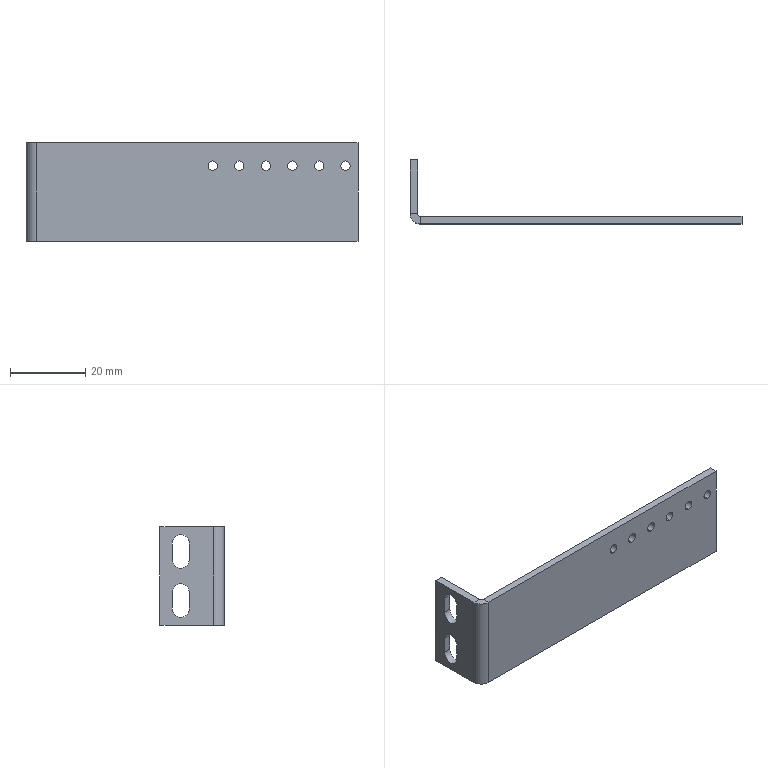Part | STEP file | 11-FG-E03211 | 1 solid | 34 faces | box 88 x 17 x 26 mm | volume 5114 mm3 | cylinder 18 | plane 16 | commonest cylinder face diameters 2.5 x12 4.5 x4 1.473 x1 5.473 x1
STEP:
#1=CARTESIAN_POINT('',(49.5,0.,18.725));
#2=VERTEX_POINT('',#1);
#3=CARTESIAN_POINT('',(49.5,0.,21.225));
#4=VERTEX_POINT('',#3);
#5=CARTESIAN_POINT('',(49.5,0.,19.975));
#6=DIRECTION('',(0.,1.,0.));
#7=DIRECTION('',(0.,0.,1.));
#8=AXIS2_PLACEMENT_3D('',#5,#6,#7);
#9=CIRCLE('',#8,1.25);
#10=EDGE_CURVE('',#2,#4,#9,.T.);
#11=ORIENTED_EDGE('',*,*,#10,.T.);
#12=CARTESIAN_POINT('',(49.5,-2.,21.225));
#13=VERTEX_POINT('',#12);
#14=CARTESIAN_POINT('',(49.5,-2.,21.225));
#15=DIRECTION('',(0.,-1.,0.));
#16=VECTOR('',#15,1000.);
#17=LINE('',#14,#16);
#18=EDGE_CURVE('',#4,#13,#17,.T.);
#19=ORIENTED_EDGE('',*,*,#18,.T.);
#20=CARTESIAN_POINT('',(49.5,-2.,18.725));
#21=VERTEX_POINT('',#20);
#22=CARTESIAN_POINT('',(49.5,-2.,19.975));
#23=DIRECTION('',(0.,-1.,0.));
#24=DIRECTION('',(0.,0.,-1.));
#25=AXIS2_PLACEMENT_3D('',#22,#23,#24);
#26=CIRCLE('',#25,1.25);
#27=EDGE_CURVE('',#13,#21,#26,.T.);
#28=ORIENTED_EDGE('',*,*,#27,.T.);
#29=CARTESIAN_POINT('',(49.5,-2.,18.725));
#30=DIRECTION('',(0.,-1.,0.));
#31=VECTOR('',#30,1000.);
#32=LINE('',#29,#31);
#33=EDGE_CURVE('',#2,#21,#32,.T.);
#34=ORIENTED_EDGE('',*,*,#33,.F.);
#35=EDGE_LOOP('',(#11,#19,#28,#34));
#36=FACE_OUTER_BOUND('',#35,.T.);
#37=CARTESIAN_POINT('',(49.5,-2.,19.975));
#38=DIRECTION('',(0.,-1.,0.));
#39=DIRECTION('',(0.,0.,-1.));
#40=AXIS2_PLACEMENT_3D('',#37,#38,#39);
#41=CYLINDRICAL_SURFACE('',#40,1.25);
#42=ADVANCED_FACE('',(#36),#41,.F.);
#43=CARTESIAN_POINT('',(56.5,0.,18.725));
#44=VERTEX_POINT('',#43);
#45=CARTESIAN_POINT('',(56.5,0.,21.225));
#46=VERTEX_POINT('',#45);
#47=CARTESIAN_POINT('',(56.5,0.,19.975));
#48=DIRECTION('',(0.,1.,0.));
#49=DIRECTION('',(0.,0.,1.));
#50=AXIS2_PLACEMENT_3D('',#47,#48,#49);
#51=CIRCLE('',#50,1.25);
#52=EDGE_CURVE('',#44,#46,#51,.T.);
#53=ORIENTED_EDGE('',*,*,#52,.T.);
#54=CARTESIAN_POINT('',(56.5,-2.,21.225));
#55=VERTEX_POINT('',#54);
#56=CARTESIAN_POINT('',(56.5,-2.,21.225));
#57=DIRECTION('',(0.,-1.,0.));
#58=VECTOR('',#57,1000.);
#59=LINE('',#56,#58);
#60=EDGE_CURVE('',#46,#55,#59,.T.);
#61=ORIENTED_EDGE('',*,*,#60,.T.);
#62=CARTESIAN_POINT('',(56.5,-2.,18.725));
#63=VERTEX_POINT('',#62);
#64=CARTESIAN_POINT('',(56.5,-2.,19.975));
#65=DIRECTION('',(0.,-1.,0.));
#66=DIRECTION('',(0.,0.,-1.));
#67=AXIS2_PLACEMENT_3D('',#64,#65,#66);
#68=CIRCLE('',#67,1.25);
#69=EDGE_CURVE('',#55,#63,#68,.T.);
#70=ORIENTED_EDGE('',*,*,#69,.T.);
#71=CARTESIAN_POINT('',(56.5,-2.,18.725));
#72=DIRECTION('',(0.,-1.,0.));
#73=VECTOR('',#72,1000.);
#74=LINE('',#71,#73);
#75=EDGE_CURVE('',#44,#63,#74,.T.);
#76=ORIENTED_EDGE('',*,*,#75,.F.);
#77=EDGE_LOOP('',(#53,#61,#70,#76));
#78=FACE_OUTER_BOUND('',#77,.T.);
#79=CARTESIAN_POINT('',(56.5,-2.,19.975));
#80=DIRECTION('',(0.,-1.,0.));
#81=DIRECTION('',(0.,0.,-1.));
#82=AXIS2_PLACEMENT_3D('',#79,#80,#81);
#83=CYLINDRICAL_SURFACE('',#82,1.25);
#84=ADVANCED_FACE('',(#78),#83,.F.);
#85=CARTESIAN_POINT('',(63.6,0.,18.725));
#86=VERTEX_POINT('',#85);
#87=CARTESIAN_POINT('',(63.6,0.,21.225));
#88=VERTEX_POINT('',#87);
#89=CARTESIAN_POINT('',(63.6,0.,19.975));
#90=DIRECTION('',(0.,1.,0.));
#91=DIRECTION('',(0.,0.,1.));
#92=AXIS2_PLACEMENT_3D('',#89,#90,#91);
#93=CIRCLE('',#92,1.25);
#94=EDGE_CURVE('',#86,#88,#93,.T.);
#95=ORIENTED_EDGE('',*,*,#94,.T.);
#96=CARTESIAN_POINT('',(63.6,-2.,21.225));
#97=VERTEX_POINT('',#96);
#98=CARTESIAN_POINT('',(63.6,-2.,21.225));
#99=DIRECTION('',(0.,-1.,0.));
#100=VECTOR('',#99,1000.);
#101=LINE('',#98,#100);
#102=EDGE_CURVE('',#88,#97,#101,.T.);
#103=ORIENTED_EDGE('',*,*,#102,.T.);
#104=CARTESIAN_POINT('',(63.6,-2.,18.725));
#105=VERTEX_POINT('',#104);
#106=CARTESIAN_POINT('',(63.6,-2.,19.975));
#107=DIRECTION('',(0.,-1.,0.));
#108=DIRECTION('',(0.,0.,-1.));
#109=AXIS2_PLACEMENT_3D('',#106,#107,#108);
#110=CIRCLE('',#109,1.25);
#111=EDGE_CURVE('',#97,#105,#110,.T.);
#112=ORIENTED_EDGE('',*,*,#111,.T.);
#113=CARTESIAN_POINT('',(63.6,-2.,18.725));
#114=DIRECTION('',(0.,-1.,0.));
#115=VECTOR('',#114,1000.);
#116=LINE('',#113,#115);
#117=EDGE_CURVE('',#86,#105,#116,.T.);
#118=ORIENTED_EDGE('',*,*,#117,.F.);
#119=EDGE_LOOP('',(#95,#103,#112,#118));
#120=FACE_OUTER_BOUND('',#119,.T.);
#121=CARTESIAN_POINT('',(63.6,-2.,19.975));
#122=DIRECTION('',(0.,-1.,0.));
#123=DIRECTION('',(0.,0.,-1.));
#124=AXIS2_PLACEMENT_3D('',#121,#122,#123);
#125=CYLINDRICAL_SURFACE('',#124,1.25);
#126=ADVANCED_FACE('',(#120),#125,.F.);
#127=CARTESIAN_POINT('',(70.6,0.,18.725));
#128=VERTEX_POINT('',#127);
#129=CARTESIAN_POINT('',(70.6,0.,21.225));
#130=VERTEX_POINT('',#129);
#131=CARTESIAN_POINT('',(70.6,0.,19.975));
#132=DIRECTION('',(0.,1.,0.));
#133=DIRECTION('',(0.,0.,1.));
#134=AXIS2_PLACEMENT_3D('',#131,#132,#133);
#135=CIRCLE('',#134,1.25);
#136=EDGE_CURVE('',#128,#130,#135,.T.);
#137=ORIENTED_EDGE('',*,*,#136,.T.);
#138=CARTESIAN_POINT('',(70.6,-2.,21.225));
#139=VERTEX_POINT('',#138);
#140=CARTESIAN_POINT('',(70.6,-2.,21.225));
#141=DIRECTION('',(0.,-1.,0.));
#142=VECTOR('',#141,1000.);
#143=LINE('',#140,#142);
#144=EDGE_CURVE('',#130,#139,#143,.T.);
#145=ORIENTED_EDGE('',*,*,#144,.T.);
#146=CARTESIAN_POINT('',(70.6,-2.,18.725));
#147=VERTEX_POINT('',#146);
#148=CARTESIAN_POINT('',(70.6,-2.,19.975));
#149=DIRECTION('',(0.,-1.,0.));
#150=DIRECTION('',(0.,0.,-1.));
#151=AXIS2_PLACEMENT_3D('',#148,#149,#150);
#152=CIRCLE('',#151,1.25);
#153=EDGE_CURVE('',#139,#147,#152,.T.);
#154=ORIENTED_EDGE('',*,*,#153,.T.);
#155=CARTESIAN_POINT('',(70.6,-2.,18.725));
#156=DIRECTION('',(0.,-1.,0.));
#157=VECTOR('',#156,1000.);
#158=LINE('',#155,#157);
#159=EDGE_CURVE('',#128,#147,#158,.T.);
#160=ORIENTED_EDGE('',*,*,#159,.F.);
#161=EDGE_LOOP('',(#137,#145,#154,#160));
#162=FACE_OUTER_BOUND('',#161,.T.);
#163=CARTESIAN_POINT('',(70.6,-2.,19.975));
#164=DIRECTION('',(0.,-1.,0.));
#165=DIRECTION('',(0.,0.,-1.));
#166=AXIS2_PLACEMENT_3D('',#163,#164,#165);
#167=CYLINDRICAL_SURFACE('',#166,1.25);
#168=ADVANCED_FACE('',(#162),#167,.F.);
#169=CARTESIAN_POINT('',(77.7,0.,18.725));
#170=VERTEX_POINT('',#169);
#171=CARTESIAN_POINT('',(77.7,0.,21.225));
#172=VERTEX_POINT('',#171);
#173=CARTESIAN_POINT('',(77.7,0.,19.975));
#174=DIRECTION('',(0.,1.,0.));
#175=DIRECTION('',(0.,0.,1.));
#176=AXIS2_PLACEMENT_3D('',#173,#174,#175);
#177=CIRCLE('',#176,1.25);
#178=EDGE_CURVE('',#170,#172,#177,.T.);
#179=ORIENTED_EDGE('',*,*,#178,.T.);
#180=CARTESIAN_POINT('',(77.7,-2.,21.225));
#181=VERTEX_POINT('',#180);
#182=CARTESIAN_POINT('',(77.7,-2.,21.225));
#183=DIRECTION('',(0.,-1.,0.));
#184=VECTOR('',#183,1000.);
#185=LINE('',#182,#184);
#186=EDGE_CURVE('',#172,#181,#185,.T.);
#187=ORIENTED_EDGE('',*,*,#186,.T.);
#188=CARTESIAN_POINT('',(77.7,-2.,18.725));
#189=VERTEX_POINT('',#188);
#190=CARTESIAN_POINT('',(77.7,-2.,19.975));
#191=DIRECTION('',(0.,-1.,0.));
#192=DIRECTION('',(0.,0.,-1.));
#193=AXIS2_PLACEMENT_3D('',#190,#191,#192);
#194=CIRCLE('',#193,1.25);
#195=EDGE_CURVE('',#181,#189,#194,.T.);
#196=ORIENTED_EDGE('',*,*,#195,.T.);
#197=CARTESIAN_POINT('',(77.7,-2.,18.725));
#198=DIRECTION('',(0.,-1.,0.));
#199=VECTOR('',#198,1000.);
#200=LINE('',#197,#199);
#201=EDGE_CURVE('',#170,#189,#200,.T.);
#202=ORIENTED_EDGE('',*,*,#201,.F.);
#203=EDGE_LOOP('',(#179,#187,#196,#202));
#204=FACE_OUTER_BOUND('',#203,.T.);
#205=CARTESIAN_POINT('',(77.7,-2.,19.975));
#206=DIRECTION('',(0.,-1.,0.));
#207=DIRECTION('',(0.,0.,-1.));
#208=AXIS2_PLACEMENT_3D('',#205,#206,#207);
#209=CYLINDRICAL_SURFACE('',#208,1.25);
#210=ADVANCED_FACE('',(#204),#209,.F.);
#211=CARTESIAN_POINT('',(84.7,0.,18.725));
#212=VERTEX_POINT('',#211);
#213=CARTESIAN_POINT('',(84.7,0.,21.225));
#214=VERTEX_POINT('',#213);
#215=CARTESIAN_POINT('',(84.7,0.,19.975));
#216=DIRECTION('',(0.,1.,0.));
#217=DIRECTION('',(0.,0.,1.));
#218=AXIS2_PLACEMENT_3D('',#215,#216,#217);
#219=CIRCLE('',#218,1.25);
#220=EDGE_CURVE('',#212,#214,#219,.T.);
#221=ORIENTED_EDGE('',*,*,#220,.T.);
#222=CARTESIAN_POINT('',(84.7,-2.,21.225));
#223=VERTEX_POINT('',#222);
#224=CARTESIAN_POINT('',(84.7,-2.,21.225));
#225=DIRECTION('',(0.,-1.,0.));
#226=VECTOR('',#225,1000.);
#227=LINE('',#224,#226);
#228=EDGE_CURVE('',#214,#223,#227,.T.);
#229=ORIENTED_EDGE('',*,*,#228,.T.);
#230=CARTESIAN_POINT('',(84.7,-2.,18.725));
#231=VERTEX_POINT('',#230);
#232=CARTESIAN_POINT('',(84.7,-2.,19.975));
#233=DIRECTION('',(0.,-1.,0.));
#234=DIRECTION('',(0.,0.,-1.));
#235=AXIS2_PLACEMENT_3D('',#232,#233,#234);
#236=CIRCLE('',#235,1.25);
#237=EDGE_CURVE('',#223,#231,#236,.T.);
#238=ORIENTED_EDGE('',*,*,#237,.T.);
#239=CARTESIAN_POINT('',(84.7,-2.,18.725));
#240=DIRECTION('',(0.,-1.,0.));
#241=VECTOR('',#240,1000.);
#242=LINE('',#239,#241);
#243=EDGE_CURVE('',#212,#231,#242,.T.);
#244=ORIENTED_EDGE('',*,*,#243,.F.);
#245=EDGE_LOOP('',(#221,#229,#238,#244));
#246=FACE_OUTER_BOUND('',#245,.T.);
#247=CARTESIAN_POINT('',(84.7,-2.,19.975));
#248=DIRECTION('',(0.,-1.,0.));
#249=DIRECTION('',(0.,0.,-1.));
#250=AXIS2_PLACEMENT_3D('',#247,#248,#249);
#251=CYLINDRICAL_SURFACE('',#250,1.25);
#252=ADVANCED_FACE('',(#246),#251,.F.);
#253=CARTESIAN_POINT('',(49.5,-2.,19.975));
#254=DIRECTION('',(0.,-1.,0.));
#255=DIRECTION('',(0.,0.,-1.));
#256=AXIS2_PLACEMENT_3D('',#253,#254,#255);
#257=CIRCLE('',#256,1.25);
#258=EDGE_CURVE('',#21,#13,#257,.T.);
#259=ORIENTED_EDGE('',*,*,#258,.F.);
#260=ORIENTED_EDGE('',*,*,#27,.F.);
#261=EDGE_LOOP('',(#259,#260));
#262=FACE_BOUND('',#261,.T.);
#263=CARTESIAN_POINT('',(56.5,-2.,19.975));
#264=DIRECTION('',(0.,-1.,0.));
#265=DIRECTION('',(0.,0.,-1.));
#266=AXIS2_PLACEMENT_3D('',#263,#264,#265);
#267=CIRCLE('',#266,1.25);
#268=EDGE_CURVE('',#63,#55,#267,.T.);
#269=ORIENTED_EDGE('',*,*,#268,.F.);
#270=ORIENTED_EDGE('',*,*,#69,.F.);
#271=EDGE_LOOP('',(#269,#270));
#272=FACE_BOUND('',#271,.T.);
#273=CARTESIAN_POINT('',(63.6,-2.,19.975));
#274=DIRECTION('',(0.,-1.,0.));
#275=DIRECTION('',(0.,0.,-1.));
#276=AXIS2_PLACEMENT_3D('',#273,#274,#275);
#277=CIRCLE('',#276,1.25);
#278=EDGE_CURVE('',#105,#97,#277,.T.);
#279=ORIENTED_EDGE('',*,*,#278,.F.);
#280=ORIENTED_EDGE('',*,*,#111,.F.);
#281=EDGE_LOOP('',(#279,#280));
#282=FACE_BOUND('',#281,.T.);
#283=CARTESIAN_POINT('',(70.6,-2.,19.975));
#284=DIRECTION('',(0.,-1.,0.));
#285=DIRECTION('',(0.,0.,-1.));
#286=AXIS2_PLACEMENT_3D('',#283,#284,#285);
#287=CIRCLE('',#286,1.25);
#288=EDGE_CURVE('',#147,#139,#287,.T.);
#289=ORIENTED_EDGE('',*,*,#288,.F.);
#290=ORIENTED_EDGE('',*,*,#153,.F.);
#291=EDGE_LOOP('',(#289,#290));
#292=FACE_BOUND('',#291,.T.);
#293=CARTESIAN_POINT('',(77.7,-2.,19.975));
#294=DIRECTION('',(0.,-1.,0.));
#295=DIRECTION('',(0.,0.,-1.));
#296=AXIS2_PLACEMENT_3D('',#293,#294,#295);
#297=CIRCLE('',#296,1.25);
#298=EDGE_CURVE('',#189,#181,#297,.T.);
#299=ORIENTED_EDGE('',*,*,#298,.F.);
#300=ORIENTED_EDGE('',*,*,#195,.F.);
#301=EDGE_LOOP('',(#299,#300));
#302=FACE_BOUND('',#301,.T.);
#303=CARTESIAN_POINT('',(84.7,-2.,19.975));
#304=DIRECTION('',(0.,-1.,0.));
#305=DIRECTION('',(0.,0.,-1.));
#306=AXIS2_PLACEMENT_3D('',#303,#304,#305);
#307=CIRCLE('',#306,1.25);
#308=EDGE_CURVE('',#231,#223,#307,.T.);
#309=ORIENTED_EDGE('',*,*,#308,.F.);
#310=ORIENTED_EDGE('',*,*,#237,.F.);
#311=EDGE_LOOP('',(#309,#310));
#312=FACE_BOUND('',#311,.T.);
#313=CARTESIAN_POINT('',(2.737,-2.,26.));
#314=VERTEX_POINT('',#313);
#315=CARTESIAN_POINT('',(2.737,-2.,0.));
#316=VERTEX_POINT('',#315);
#317=CARTESIAN_POINT('',(2.737,-2.,26.));
#318=DIRECTION('',(0.,0.,-1.));
#319=VECTOR('',#318,1000.);
#320=LINE('',#317,#319);
#321=EDGE_CURVE('',#314,#316,#320,.T.);
#322=ORIENTED_EDGE('',*,*,#321,.T.);
#323=CARTESIAN_POINT('',(88.,-2.,0.));
#324=VERTEX_POINT('',#323);
#325=CARTESIAN_POINT('',(0.,-2.,0.));
#326=DIRECTION('',(1.,0.,0.));
#327=VECTOR('',#326,1000.);
#328=LINE('',#325,#327);
#329=EDGE_CURVE('',#316,#324,#328,.T.);
#330=ORIENTED_EDGE('',*,*,#329,.T.);
#331=CARTESIAN_POINT('',(88.,-2.,26.));
#332=VERTEX_POINT('',#331);
#333=CARTESIAN_POINT('',(88.,-2.,26.));
#334=DIRECTION('',(0.,0.,-1.));
#335=VECTOR('',#334,1000.);
#336=LINE('',#333,#335);
#337=EDGE_CURVE('',#332,#324,#336,.T.);
#338=ORIENTED_EDGE('',*,*,#337,.F.);
#339=CARTESIAN_POINT('',(0.,-2.,26.));
#340=DIRECTION('',(1.,0.,0.));
#341=VECTOR('',#340,1000.);
#342=LINE('',#339,#341);
#343=EDGE_CURVE('',#314,#332,#342,.T.);
#344=ORIENTED_EDGE('',*,*,#343,.F.);
#345=EDGE_LOOP('',(#322,#330,#338,#344));
#346=FACE_OUTER_BOUND('',#345,.T.);
#347=CARTESIAN_POINT('',(0.,-2.,26.));
#348=DIRECTION('',(0.,1.,0.));
#349=DIRECTION('',(0.,0.,1.));
#350=AXIS2_PLACEMENT_3D('',#347,#348,#349);
#351=PLANE('',#350);
#352=ADVANCED_FACE('',(#262,#272,#282,#292,#302,#312,#346),#351,.F.);
#353=ORIENTED_EDGE('',*,*,#10,.F.);
#354=CARTESIAN_POINT('',(49.5,0.,19.975));
#355=DIRECTION('',(0.,1.,0.));
#356=DIRECTION('',(0.,0.,1.));
#357=AXIS2_PLACEMENT_3D('',#354,#355,#356);
#358=CIRCLE('',#357,1.25);
#359=EDGE_CURVE('',#4,#2,#358,.T.);
#360=ORIENTED_EDGE('',*,*,#359,.F.);
#361=EDGE_LOOP('',(#353,#360));
#362=FACE_BOUND('',#361,.T.);
#363=ORIENTED_EDGE('',*,*,#52,.F.);
#364=CARTESIAN_POINT('',(56.5,0.,19.975));
#365=DIRECTION('',(0.,1.,0.));
#366=DIRECTION('',(0.,0.,1.));
#367=AXIS2_PLACEMENT_3D('',#364,#365,#366);
#368=CIRCLE('',#367,1.25);
#369=EDGE_CURVE('',#46,#44,#368,.T.);
#370=ORIENTED_EDGE('',*,*,#369,.F.);
#371=EDGE_LOOP('',(#363,#370));
#372=FACE_BOUND('',#371,.T.);
#373=ORIENTED_EDGE('',*,*,#94,.F.);
#374=CARTESIAN_POINT('',(63.6,0.,19.975));
#375=DIRECTION('',(0.,1.,0.));
#376=DIRECTION('',(0.,0.,1.));
#377=AXIS2_PLACEMENT_3D('',#374,#375,#376);
#378=CIRCLE('',#377,1.25);
#379=EDGE_CURVE('',#88,#86,#378,.T.);
#380=ORIENTED_EDGE('',*,*,#379,.F.);
#381=EDGE_LOOP('',(#373,#380));
#382=FACE_BOUND('',#381,.T.);
#383=ORIENTED_EDGE('',*,*,#136,.F.);
#384=CARTESIAN_POINT('',(70.6,0.,19.975));
#385=DIRECTION('',(0.,1.,0.));
#386=DIRECTION('',(0.,0.,1.));
#387=AXIS2_PLACEMENT_3D('',#384,#385,#386);
#388=CIRCLE('',#387,1.25);
#389=EDGE_CURVE('',#130,#128,#388,.T.);
#390=ORIENTED_EDGE('',*,*,#389,.F.);
#391=EDGE_LOOP('',(#383,#390));
#392=FACE_BOUND('',#391,.T.);
#393=ORIENTED_EDGE('',*,*,#178,.F.);
#394=CARTESIAN_POINT('',(77.7,0.,19.975));
#395=DIRECTION('',(0.,1.,0.));
#396=DIRECTION('',(0.,0.,1.));
#397=AXIS2_PLACEMENT_3D('',#394,#395,#396);
#398=CIRCLE('',#397,1.25);
#399=EDGE_CURVE('',#172,#170,#398,.T.);
#400=ORIENTED_EDGE('',*,*,#399,.F.);
#401=EDGE_LOOP('',(#393,#400));
#402=FACE_BOUND('',#401,.T.);
#403=ORIENTED_EDGE('',*,*,#220,.F.);
#404=CARTESIAN_POINT('',(84.7,0.,19.975));
#405=DIRECTION('',(0.,1.,0.));
#406=DIRECTION('',(0.,0.,1.));
#407=AXIS2_PLACEMENT_3D('',#404,#405,#406);
#408=CIRCLE('',#407,1.25);
#409=EDGE_CURVE('',#214,#212,#408,.T.);
#410=ORIENTED_EDGE('',*,*,#409,.F.);
#411=EDGE_LOOP('',(#403,#410));
#412=FACE_BOUND('',#411,.T.);
#413=CARTESIAN_POINT('',(2.737,0.,0.));
#414=VERTEX_POINT('',#413);
#415=CARTESIAN_POINT('',(88.,0.,0.));
#416=VERTEX_POINT('',#415);
#417=CARTESIAN_POINT('',(0.,0.,0.));
#418=DIRECTION('',(1.,0.,0.));
#419=VECTOR('',#418,1000.);
#420=LINE('',#417,#419);
#421=EDGE_CURVE('',#414,#416,#420,.T.);
#422=ORIENTED_EDGE('',*,*,#421,.F.);
#423=CARTESIAN_POINT('',(2.737,0.,26.));
#424=VERTEX_POINT('',#423);
#425=CARTESIAN_POINT('',(2.737,0.,26.));
#426=DIRECTION('',(0.,0.,-1.));
#427=VECTOR('',#426,1000.);
#428=LINE('',#425,#427);
#429=EDGE_CURVE('',#424,#414,#428,.T.);
#430=ORIENTED_EDGE('',*,*,#429,.F.);
#431=CARTESIAN_POINT('',(88.,0.,26.));
#432=VERTEX_POINT('',#431);
#433=CARTESIAN_POINT('',(0.,0.,26.));
#434=DIRECTION('',(1.,0.,0.));
#435=VECTOR('',#434,1000.);
#436=LINE('',#433,#435);
#437=EDGE_CURVE('',#424,#432,#436,.T.);
#438=ORIENTED_EDGE('',*,*,#437,.T.);
#439=CARTESIAN_POINT('',(88.,0.,26.));
#440=DIRECTION('',(0.,0.,-1.));
#441=VECTOR('',#440,1000.);
#442=LINE('',#439,#441);
#443=EDGE_CURVE('',#432,#416,#442,.T.);
#444=ORIENTED_EDGE('',*,*,#443,.T.);
#445=EDGE_LOOP('',(#422,#430,#438,#444));
#446=FACE_OUTER_BOUND('',#445,.T.);
#447=CARTESIAN_POINT('',(0.,0.,26.));
#448=DIRECTION('',(0.,1.,0.));
#449=DIRECTION('',(0.,0.,1.));
#450=AXIS2_PLACEMENT_3D('',#447,#448,#449);
#451=PLANE('',#450);
#452=ADVANCED_FACE('',(#362,#372,#382,#392,#402,#412,#446),#451,.T.);
#453=CARTESIAN_POINT('',(2.737,0.,26.));
#454=DIRECTION('',(0.,-1.,0.));
#455=VECTOR('',#454,1000.);
#456=LINE('',#453,#455);
#457=EDGE_CURVE('',#424,#314,#456,.T.);
#458=ORIENTED_EDGE('',*,*,#457,.T.);
#459=ORIENTED_EDGE('',*,*,#343,.T.);
#460=CARTESIAN_POINT('',(88.,0.,26.));
#461=DIRECTION('',(0.,-1.,0.));
#462=VECTOR('',#461,1000.);
#463=LINE('',#460,#462);
#464=EDGE_CURVE('',#432,#332,#463,.T.);
#465=ORIENTED_EDGE('',*,*,#464,.F.);
#466=ORIENTED_EDGE('',*,*,#437,.F.);
#467=EDGE_LOOP('',(#458,#459,#465,#466));
#468=FACE_OUTER_BOUND('',#467,.T.);
#469=CARTESIAN_POINT('',(0.,0.,26.));
#470=DIRECTION('',(0.,0.,-1.));
#471=DIRECTION('',(-1.,0.,0.));
#472=AXIS2_PLACEMENT_3D('',#469,#470,#471);
#473=PLANE('',#472);
#474=ADVANCED_FACE('',(#468),#473,.F.);
#475=CARTESIAN_POINT('',(88.,0.,0.));
#476=DIRECTION('',(0.,-1.,0.));
#477=VECTOR('',#476,1000.);
#478=LINE('',#475,#477);
#479=EDGE_CURVE('',#416,#324,#478,.T.);
#480=ORIENTED_EDGE('',*,*,#479,.F.);
#481=ORIENTED_EDGE('',*,*,#443,.F.);
#482=ORIENTED_EDGE('',*,*,#464,.T.);
#483=ORIENTED_EDGE('',*,*,#337,.T.);
#484=EDGE_LOOP('',(#480,#481,#482,#483));
#485=FACE_OUTER_BOUND('',#484,.T.);
#486=CARTESIAN_POINT('',(88.,0.,26.));
#487=DIRECTION('',(1.,0.,0.));
#488=DIRECTION('',(0.,0.,-1.));
#489=AXIS2_PLACEMENT_3D('',#486,#487,#488);
#490=PLANE('',#489);
#491=ADVANCED_FACE('',(#485),#490,.T.);
#492=CARTESIAN_POINT('',(2.737,0.,0.));
#493=DIRECTION('',(0.,-1.,0.));
#494=VECTOR('',#493,1000.);
#495=LINE('',#492,#494);
#496=EDGE_CURVE('',#414,#316,#495,.T.);
#497=ORIENTED_EDGE('',*,*,#496,.F.);
#498=ORIENTED_EDGE('',*,*,#421,.T.);
#499=ORIENTED_EDGE('',*,*,#479,.T.);
#500=ORIENTED_EDGE('',*,*,#329,.F.);
#501=EDGE_LOOP('',(#497,#498,#499,#500));
#502=FACE_OUTER_BOUND('',#501,.T.);
#503=CARTESIAN_POINT('',(0.,0.,0.));
#504=DIRECTION('',(0.,0.,-1.));
#505=DIRECTION('',(-1.,0.,0.));
#506=AXIS2_PLACEMENT_3D('',#503,#504,#505);
#507=PLANE('',#506);
#508=ADVANCED_FACE('',(#502),#507,.T.);
#509=CARTESIAN_POINT('',(2.,0.7366,0.));
#510=VERTEX_POINT('',#509);
#511=CARTESIAN_POINT('',(0.,0.7366,0.));
#512=VERTEX_POINT('',#511);
#513=CARTESIAN_POINT('',(0.,0.7366,0.));
#514=DIRECTION('',(-1.,0.,0.));
#515=VECTOR('',#514,1000.);
#516=LINE('',#513,#515);
#517=EDGE_CURVE('',#510,#512,#516,.T.);
#518=ORIENTED_EDGE('',*,*,#517,.F.);
#519=CARTESIAN_POINT('',(2.737,0.7366,0.));
#520=DIRECTION('',(0.,0.,-1.));
#521=DIRECTION('',(1.,0.,0.));
#522=AXIS2_PLACEMENT_3D('',#519,#520,#521);
#523=CIRCLE('',#522,0.7366);
#524=EDGE_CURVE('',#414,#510,#523,.T.);
#525=ORIENTED_EDGE('',*,*,#524,.F.);
#526=ORIENTED_EDGE('',*,*,#496,.T.);
#527=CARTESIAN_POINT('',(2.737,0.7366,0.));
#528=DIRECTION('',(0.,0.,-1.));
#529=DIRECTION('',(1.,0.,0.));
#530=AXIS2_PLACEMENT_3D('',#527,#528,#529);
#531=CIRCLE('',#530,2.737);
#532=EDGE_CURVE('',#316,#512,#531,.T.);
#533=ORIENTED_EDGE('',*,*,#532,.T.);
#534=EDGE_LOOP('',(#518,#525,#526,#533));
#535=FACE_OUTER_BOUND('',#534,.T.);
#536=CARTESIAN_POINT('',(2.737,0.7366,0.));
#537=DIRECTION('',(0.,0.,-1.));
#538=DIRECTION('',(-1.,0.,0.));
#539=AXIS2_PLACEMENT_3D('',#536,#537,#538);
#540=PLANE('',#539);
#541=ADVANCED_FACE('',(#535),#540,.T.);
#542=CARTESIAN_POINT('',(2.,0.7366,26.));
#543=VERTEX_POINT('',#542);
#544=CARTESIAN_POINT('',(2.737,0.7366,26.));
#545=DIRECTION('',(0.,0.,1.));
#546=DIRECTION('',(1.,0.,0.));
#547=AXIS2_PLACEMENT_3D('',#544,#545,#546);
#548=CIRCLE('',#547,0.7366);
#549=EDGE_CURVE('',#543,#424,#548,.T.);
#550=ORIENTED_EDGE('',*,*,#549,.F.);
#551=CARTESIAN_POINT('',(0.,0.7366,26.));
#552=VERTEX_POINT('',#551);
#553=CARTESIAN_POINT('',(2.,0.7366,26.));
#554=DIRECTION('',(-1.,0.,0.));
#555=VECTOR('',#554,1000.);
#556=LINE('',#553,#555);
#557=EDGE_CURVE('',#543,#552,#556,.T.);
#558=ORIENTED_EDGE('',*,*,#557,.T.);
#559=CARTESIAN_POINT('',(2.737,0.7366,26.));
#560=DIRECTION('',(0.,0.,1.));
#561=DIRECTION('',(1.,0.,0.));
#562=AXIS2_PLACEMENT_3D('',#559,#560,#561);
#563=CIRCLE('',#562,2.737);
#564=EDGE_CURVE('',#552,#314,#563,.T.);
#565=ORIENTED_EDGE('',*,*,#564,.T.);
#566=ORIENTED_EDGE('',*,*,#457,.F.);
#567=EDGE_LOOP('',(#550,#558,#565,#566));
#568=FACE_OUTER_BOUND('',#567,.T.);
#569=CARTESIAN_POINT('',(2.737,0.7366,26.));
#570=DIRECTION('',(0.,0.,-1.));
#571=DIRECTION('',(-1.,0.,0.));
#572=AXIS2_PLACEMENT_3D('',#569,#570,#571);
#573=PLANE('',#572);
#574=ADVANCED_FACE('',(#568),#573,.F.);
#575=ORIENTED_EDGE('',*,*,#321,.F.);
#576=ORIENTED_EDGE('',*,*,#564,.F.);
#577=CARTESIAN_POINT('',(0.,0.7366,0.));
#578=DIRECTION('',(0.,0.,1.));
#579=VECTOR('',#578,1000.);
#580=LINE('',#577,#579);
#581=EDGE_CURVE('',#512,#552,#580,.T.);
#582=ORIENTED_EDGE('',*,*,#581,.F.);
#583=ORIENTED_EDGE('',*,*,#532,.F.);
#584=EDGE_LOOP('',(#575,#576,#582,#583));
#585=FACE_OUTER_BOUND('',#584,.T.);
#586=CARTESIAN_POINT('',(2.737,0.7366,26.));
#587=DIRECTION('',(0.,0.,1.));
#588=DIRECTION('',(-1.,0.,0.));
#589=AXIS2_PLACEMENT_3D('',#586,#587,#588);
#590=CYLINDRICAL_SURFACE('',#589,2.737);
#591=ADVANCED_FACE('',(#585),#590,.T.);
#592=ORIENTED_EDGE('',*,*,#429,.T.);
#593=ORIENTED_EDGE('',*,*,#524,.T.);
#594=CARTESIAN_POINT('',(2.,0.7366,0.));
#595=DIRECTION('',(0.,0.,1.));
#596=VECTOR('',#595,1000.);
#597=LINE('',#594,#596);
#598=EDGE_CURVE('',#510,#543,#597,.T.);
#599=ORIENTED_EDGE('',*,*,#598,.T.);
#600=ORIENTED_EDGE('',*,*,#549,.T.);
#601=EDGE_LOOP('',(#592,#593,#599,#600));
#602=FACE_OUTER_BOUND('',#601,.T.);
#603=CARTESIAN_POINT('',(2.737,0.7366,26.));
#604=DIRECTION('',(0.,0.,1.));
#605=DIRECTION('',(-1.,0.,0.));
#606=AXIS2_PLACEMENT_3D('',#603,#604,#605);
#607=CYLINDRICAL_SURFACE('',#606,0.7366);
#608=ADVANCED_FACE('',(#602),#607,.F.);
#609=CARTESIAN_POINT('',(0.,15.,26.));
#610=VERTEX_POINT('',#609);
#611=CARTESIAN_POINT('',(0.,0.,26.));
#612=DIRECTION('',(0.,-1.,0.));
#613=VECTOR('',#612,1000.);
#614=LINE('',#611,#613);
#615=EDGE_CURVE('',#610,#552,#614,.T.);
#616=ORIENTED_EDGE('',*,*,#615,.T.);
#617=ORIENTED_EDGE('',*,*,#557,.F.);
#618=CARTESIAN_POINT('',(2.,15.,26.));
#619=VERTEX_POINT('',#618);
#620=CARTESIAN_POINT('',(2.,0.,26.));
#621=DIRECTION('',(0.,-1.,0.));
#622=VECTOR('',#621,1000.);
#623=LINE('',#620,#622);
#624=EDGE_CURVE('',#619,#543,#623,.T.);
#625=ORIENTED_EDGE('',*,*,#624,.F.);
#626=CARTESIAN_POINT('',(0.,15.,26.));
#627=DIRECTION('',(1.,0.,0.));
#628=VECTOR('',#627,1000.);
#629=LINE('',#626,#628);
#630=EDGE_CURVE('',#610,#619,#629,.T.);
#631=ORIENTED_EDGE('',*,*,#630,.F.);
#632=EDGE_LOOP('',(#616,#617,#625,#631));
#633=FACE_OUTER_BOUND('',#632,.T.);
#634=CARTESIAN_POINT('',(0.,0.,26.));
#635=DIRECTION('',(0.,0.,1.));
#636=DIRECTION('',(0.,-1.,0.));
#637=AXIS2_PLACEMENT_3D('',#634,#635,#636);
#638=PLANE('',#637);
#639=ADVANCED_FACE('',(#633),#638,.T.);
#640=CARTESIAN_POINT('',(2.,15.,0.));
#641=VERTEX_POINT('',#640);
#642=CARTESIAN_POINT('',(2.,0.,0.));
#643=DIRECTION('',(0.,1.,0.));
#644=VECTOR('',#643,1000.);
#645=LINE('',#642,#644);
#646=EDGE_CURVE('',#510,#641,#645,.T.);
#647=ORIENTED_EDGE('',*,*,#646,.F.);
#648=ORIENTED_EDGE('',*,*,#517,.T.);
#649=CARTESIAN_POINT('',(0.,15.,0.));
#650=VERTEX_POINT('',#649);
#651=CARTESIAN_POINT('',(0.,15.,0.));
#652=DIRECTION('',(0.,1.,0.));
#653=VECTOR('',#652,1000.);
#654=LINE('',#651,#653);
#655=EDGE_CURVE('',#512,#650,#654,.T.);
#656=ORIENTED_EDGE('',*,*,#655,.T.);
#657=CARTESIAN_POINT('',(0.,15.,0.));
#658=DIRECTION('',(1.,0.,0.));
#659=VECTOR('',#658,1000.);
#660=LINE('',#657,#659);
#661=EDGE_CURVE('',#650,#641,#660,.T.);
#662=ORIENTED_EDGE('',*,*,#661,.T.);
#663=EDGE_LOOP('',(#647,#648,#656,#662));
#664=FACE_OUTER_BOUND('',#663,.T.);
#665=CARTESIAN_POINT('',(0.,15.,0.));
#666=DIRECTION('',(0.,0.,-1.));
#667=DIRECTION('',(0.,1.,0.));
#668=AXIS2_PLACEMENT_3D('',#665,#666,#667);
#669=PLANE('',#668);
#670=ADVANCED_FACE('',(#664),#669,.T.);
#671=CARTESIAN_POINT('',(0.,7.25,8.75));
#672=VERTEX_POINT('',#671);
#673=CARTESIAN_POINT('',(0.,11.75,8.75));
#674=VERTEX_POINT('',#673);
#675=CARTESIAN_POINT('',(0.,9.5,8.75));
#676=DIRECTION('',(-1.,0.,0.));
#677=DIRECTION('',(0.,-1.,0.));
#678=AXIS2_PLACEMENT_3D('',#675,#676,#677);
#679=CIRCLE('',#678,2.25);
#680=EDGE_CURVE('',#672,#674,#679,.T.);
#681=ORIENTED_EDGE('',*,*,#680,.F.);
#682=CARTESIAN_POINT('',(0.,7.25,4.25));
#683=VERTEX_POINT('',#682);
#684=CARTESIAN_POINT('',(0.,7.25,0.));
#685=DIRECTION('',(0.,0.,1.));
#686=VECTOR('',#685,1000.);
#687=LINE('',#684,#686);
#688=EDGE_CURVE('',#683,#672,#687,.T.);
#689=ORIENTED_EDGE('',*,*,#688,.F.);
#690=CARTESIAN_POINT('',(0.,11.75,4.25));
#691=VERTEX_POINT('',#690);
#692=CARTESIAN_POINT('',(0.,9.5,4.25));
#693=DIRECTION('',(-1.,0.,0.));
#694=DIRECTION('',(0.,-1.,0.));
#695=AXIS2_PLACEMENT_3D('',#692,#693,#694);
#696=CIRCLE('',#695,2.25);
#697=EDGE_CURVE('',#691,#683,#696,.T.);
#698=ORIENTED_EDGE('',*,*,#697,.F.);
#699=CARTESIAN_POINT('',(0.,11.75,0.));
#700=DIRECTION('',(0.,0.,-1.));
#701=VECTOR('',#700,1000.);
#702=LINE('',#699,#701);
#703=EDGE_CURVE('',#674,#691,#702,.T.);
#704=ORIENTED_EDGE('',*,*,#703,.F.);
#705=EDGE_LOOP('',(#681,#689,#698,#704));
#706=FACE_BOUND('',#705,.T.);
#707=CARTESIAN_POINT('',(0.,7.25,21.75));
#708=VERTEX_POINT('',#707);
#709=CARTESIAN_POINT('',(0.,11.75,21.75));
#710=VERTEX_POINT('',#709);
#711=CARTESIAN_POINT('',(0.,9.5,21.75));
#712=DIRECTION('',(-1.,0.,0.));
#713=DIRECTION('',(0.,-1.,0.));
#714=AXIS2_PLACEMENT_3D('',#711,#712,#713);
#715=CIRCLE('',#714,2.25);
#716=EDGE_CURVE('',#708,#710,#715,.T.);
#717=ORIENTED_EDGE('',*,*,#716,.F.);
#718=CARTESIAN_POINT('',(0.,7.25,17.25));
#719=VERTEX_POINT('',#718);
#720=CARTESIAN_POINT('',(0.,7.25,0.));
#721=DIRECTION('',(0.,0.,1.));
#722=VECTOR('',#721,1000.);
#723=LINE('',#720,#722);
#724=EDGE_CURVE('',#719,#708,#723,.T.);
#725=ORIENTED_EDGE('',*,*,#724,.F.);
#726=CARTESIAN_POINT('',(0.,11.75,17.25));
#727=VERTEX_POINT('',#726);
#728=CARTESIAN_POINT('',(0.,9.5,17.25));
#729=DIRECTION('',(-1.,0.,0.));
#730=DIRECTION('',(0.,-1.,0.));
#731=AXIS2_PLACEMENT_3D('',#728,#729,#730);
#732=CIRCLE('',#731,2.25);
#733=EDGE_CURVE('',#727,#719,#732,.T.);
#734=ORIENTED_EDGE('',*,*,#733,.F.);
#735=CARTESIAN_POINT('',(0.,11.75,0.));
#736=DIRECTION('',(0.,0.,-1.));
#737=VECTOR('',#736,1000.);
#738=LINE('',#735,#737);
#739=EDGE_CURVE('',#710,#727,#738,.T.);
#740=ORIENTED_EDGE('',*,*,#739,.F.);
#741=EDGE_LOOP('',(#717,#725,#734,#740));
#742=FACE_BOUND('',#741,.T.);
#743=ORIENTED_EDGE('',*,*,#655,.F.);
#744=ORIENTED_EDGE('',*,*,#581,.T.);
#745=ORIENTED_EDGE('',*,*,#615,.F.);
#746=CARTESIAN_POINT('',(0.,15.,26.));
#747=DIRECTION('',(0.,0.,1.));
#748=VECTOR('',#747,1000.);
#749=LINE('',#746,#748);
#750=EDGE_CURVE('',#650,#610,#749,.T.);
#751=ORIENTED_EDGE('',*,*,#750,.F.);
#752=EDGE_LOOP('',(#743,#744,#745,#751));
#753=FACE_OUTER_BOUND('',#752,.T.);
#754=CARTESIAN_POINT('',(0.,0.,0.));
#755=DIRECTION('',(-1.,0.,0.));
#756=DIRECTION('',(0.,-1.,0.));
#757=AXIS2_PLACEMENT_3D('',#754,#755,#756);
#758=PLANE('',#757);
#759=ADVANCED_FACE('',(#706,#742,#753),#758,.T.);
#760=CARTESIAN_POINT('',(2.,7.25,8.75));
#761=VERTEX_POINT('',#760);
#762=CARTESIAN_POINT('',(2.,7.25,4.25));
#763=VERTEX_POINT('',#762);
#764=CARTESIAN_POINT('',(2.,7.25,8.75));
#765=DIRECTION('',(0.,0.,-1.));
#766=VECTOR('',#765,1000.);
#767=LINE('',#764,#766);
#768=EDGE_CURVE('',#761,#763,#767,.T.);
#769=ORIENTED_EDGE('',*,*,#768,.F.);
#770=CARTESIAN_POINT('',(2.,11.75,8.75));
#771=VERTEX_POINT('',#770);
#772=CARTESIAN_POINT('',(2.,9.5,8.75));
#773=DIRECTION('',(1.,0.,0.));
#774=DIRECTION('',(0.,1.,0.));
#775=AXIS2_PLACEMENT_3D('',#772,#773,#774);
#776=CIRCLE('',#775,2.25);
#777=EDGE_CURVE('',#771,#761,#776,.T.);
#778=ORIENTED_EDGE('',*,*,#777,.F.);
#779=CARTESIAN_POINT('',(2.,11.75,4.25));
#780=VERTEX_POINT('',#779);
#781=CARTESIAN_POINT('',(2.,11.75,8.75));
#782=DIRECTION('',(0.,0.,1.));
#783=VECTOR('',#782,1000.);
#784=LINE('',#781,#783);
#785=EDGE_CURVE('',#780,#771,#784,.T.);
#786=ORIENTED_EDGE('',*,*,#785,.F.);
#787=CARTESIAN_POINT('',(2.,9.5,4.25));
#788=DIRECTION('',(1.,0.,0.));
#789=DIRECTION('',(0.,1.,0.));
#790=AXIS2_PLACEMENT_3D('',#787,#788,#789);
#791=CIRCLE('',#790,2.25);
#792=EDGE_CURVE('',#763,#780,#791,.T.);
#793=ORIENTED_EDGE('',*,*,#792,.F.);
#794=EDGE_LOOP('',(#769,#778,#786,#793));
#795=FACE_BOUND('',#794,.T.);
#796=CARTESIAN_POINT('',(2.,7.25,21.75));
#797=VERTEX_POINT('',#796);
#798=CARTESIAN_POINT('',(2.,7.25,17.25));
#799=VERTEX_POINT('',#798);
#800=CARTESIAN_POINT('',(2.,7.25,21.75));
#801=DIRECTION('',(0.,0.,-1.));
#802=VECTOR('',#801,1000.);
#803=LINE('',#800,#802);
#804=EDGE_CURVE('',#797,#799,#803,.T.);
#805=ORIENTED_EDGE('',*,*,#804,.F.);
#806=CARTESIAN_POINT('',(2.,11.75,21.75));
#807=VERTEX_POINT('',#806);
#808=CARTESIAN_POINT('',(2.,9.5,21.75));
#809=DIRECTION('',(1.,0.,0.));
#810=DIRECTION('',(0.,1.,0.));
#811=AXIS2_PLACEMENT_3D('',#808,#809,#810);
#812=CIRCLE('',#811,2.25);
#813=EDGE_CURVE('',#807,#797,#812,.T.);
#814=ORIENTED_EDGE('',*,*,#813,.F.);
#815=CARTESIAN_POINT('',(2.,11.75,17.25));
#816=VERTEX_POINT('',#815);
#817=CARTESIAN_POINT('',(2.,11.75,21.75));
#818=DIRECTION('',(0.,0.,1.));
#819=VECTOR('',#818,1000.);
#820=LINE('',#817,#819);
#821=EDGE_CURVE('',#816,#807,#820,.T.);
#822=ORIENTED_EDGE('',*,*,#821,.F.);
#823=CARTESIAN_POINT('',(2.,9.5,17.25));
#824=DIRECTION('',(1.,0.,0.));
#825=DIRECTION('',(0.,1.,0.));
#826=AXIS2_PLACEMENT_3D('',#823,#824,#825);
#827=CIRCLE('',#826,2.25);
#828=EDGE_CURVE('',#799,#816,#827,.T.);
#829=ORIENTED_EDGE('',*,*,#828,.F.);
#830=EDGE_LOOP('',(#805,#814,#822,#829));
#831=FACE_BOUND('',#830,.T.);
#832=ORIENTED_EDGE('',*,*,#598,.F.);
#833=ORIENTED_EDGE('',*,*,#646,.T.);
#834=CARTESIAN_POINT('',(2.,15.,0.));
#835=DIRECTION('',(0.,0.,1.));
#836=VECTOR('',#835,1000.);
#837=LINE('',#834,#836);
#838=EDGE_CURVE('',#641,#619,#837,.T.);
#839=ORIENTED_EDGE('',*,*,#838,.T.);
#840=ORIENTED_EDGE('',*,*,#624,.T.);
#841=EDGE_LOOP('',(#832,#833,#839,#840));
#842=FACE_OUTER_BOUND('',#841,.T.);
#843=CARTESIAN_POINT('',(2.,0.,0.));
#844=DIRECTION('',(-1.,0.,0.));
#845=DIRECTION('',(0.,-1.,0.));
#846=AXIS2_PLACEMENT_3D('',#843,#844,#845);
#847=PLANE('',#846);
#848=ADVANCED_FACE('',(#795,#831,#842),#847,.F.);
#849=ORIENTED_EDGE('',*,*,#838,.F.);
#850=ORIENTED_EDGE('',*,*,#661,.F.);
#851=ORIENTED_EDGE('',*,*,#750,.T.);
#852=ORIENTED_EDGE('',*,*,#630,.T.);
#853=EDGE_LOOP('',(#849,#850,#851,#852));
#854=FACE_OUTER_BOUND('',#853,.T.);
#855=CARTESIAN_POINT('',(0.,15.,26.));
#856=DIRECTION('',(0.,1.,0.));
#857=DIRECTION('',(-1.,0.,0.));
#858=AXIS2_PLACEMENT_3D('',#855,#856,#857);
#859=PLANE('',#858);
#860=ADVANCED_FACE('',(#854),#859,.T.);
#861=ORIENTED_EDGE('',*,*,#716,.T.);
#862=CARTESIAN_POINT('',(-8.,11.75,21.75));
#863=DIRECTION('',(1.,0.,0.));
#864=VECTOR('',#863,1000.);
#865=LINE('',#862,#864);
#866=EDGE_CURVE('',#710,#807,#865,.T.);
#867=ORIENTED_EDGE('',*,*,#866,.T.);
#868=ORIENTED_EDGE('',*,*,#813,.T.);
#869=CARTESIAN_POINT('',(-8.,7.25,21.75));
#870=DIRECTION('',(1.,0.,0.));
#871=VECTOR('',#870,1000.);
#872=LINE('',#869,#871);
#873=EDGE_CURVE('',#708,#797,#872,.T.);
#874=ORIENTED_EDGE('',*,*,#873,.F.);
#875=EDGE_LOOP('',(#861,#867,#868,#874));
#876=FACE_OUTER_BOUND('',#875,.T.);
#877=CARTESIAN_POINT('',(-8.,9.5,21.75));
#878=DIRECTION('',(1.,0.,0.));
#879=DIRECTION('',(0.,1.,0.));
#880=AXIS2_PLACEMENT_3D('',#877,#878,#879);
#881=CYLINDRICAL_SURFACE('',#880,2.25);
#882=ADVANCED_FACE('',(#876),#881,.F.);
#883=ORIENTED_EDGE('',*,*,#739,.T.);
#884=CARTESIAN_POINT('',(-8.,11.75,17.25));
#885=DIRECTION('',(1.,0.,0.));
#886=VECTOR('',#885,1000.);
#887=LINE('',#884,#886);
#888=EDGE_CURVE('',#727,#816,#887,.T.);
#889=ORIENTED_EDGE('',*,*,#888,.T.);
#890=ORIENTED_EDGE('',*,*,#821,.T.);
#891=ORIENTED_EDGE('',*,*,#866,.F.);
#892=EDGE_LOOP('',(#883,#889,#890,#891));
#893=FACE_OUTER_BOUND('',#892,.T.);
#894=CARTESIAN_POINT('',(-8.,11.75,21.75));
#895=DIRECTION('',(0.,1.,0.));
#896=DIRECTION('',(-1.,0.,0.));
#897=AXIS2_PLACEMENT_3D('',#894,#895,#896);
#898=PLANE('',#897);
#899=ADVANCED_FACE('',(#893),#898,.F.);
#900=ORIENTED_EDGE('',*,*,#733,.T.);
#901=CARTESIAN_POINT('',(-8.,7.25,17.25));
#902=DIRECTION('',(1.,0.,0.));
#903=VECTOR('',#902,1000.);
#904=LINE('',#901,#903);
#905=EDGE_CURVE('',#719,#799,#904,.T.);
#906=ORIENTED_EDGE('',*,*,#905,.T.);
#907=ORIENTED_EDGE('',*,*,#828,.T.);
#908=ORIENTED_EDGE('',*,*,#888,.F.);
#909=EDGE_LOOP('',(#900,#906,#907,#908));
#910=FACE_OUTER_BOUND('',#909,.T.);
#911=CARTESIAN_POINT('',(-8.,9.5,17.25));
#912=DIRECTION('',(1.,0.,0.));
#913=DIRECTION('',(0.,1.,0.));
#914=AXIS2_PLACEMENT_3D('',#911,#912,#913);
#915=CYLINDRICAL_SURFACE('',#914,2.25);
#916=ADVANCED_FACE('',(#910),#915,.F.);
#917=ORIENTED_EDGE('',*,*,#724,.T.);
#918=ORIENTED_EDGE('',*,*,#873,.T.);
#919=ORIENTED_EDGE('',*,*,#804,.T.);
#920=ORIENTED_EDGE('',*,*,#905,.F.);
#921=EDGE_LOOP('',(#917,#918,#919,#920));
#922=FACE_OUTER_BOUND('',#921,.T.);
#923=CARTESIAN_POINT('',(-8.,7.25,21.75));
#924=DIRECTION('',(0.,-1.,0.));
#925=DIRECTION('',(1.,0.,0.));
#926=AXIS2_PLACEMENT_3D('',#923,#924,#925);
#927=PLANE('',#926);
#928=ADVANCED_FACE('',(#922),#927,.F.);
#929=ORIENTED_EDGE('',*,*,#680,.T.);
#930=CARTESIAN_POINT('',(-8.,11.75,8.75));
#931=DIRECTION('',(1.,0.,0.));
#932=VECTOR('',#931,1000.);
#933=LINE('',#930,#932);
#934=EDGE_CURVE('',#674,#771,#933,.T.);
#935=ORIENTED_EDGE('',*,*,#934,.T.);
#936=ORIENTED_EDGE('',*,*,#777,.T.);
#937=CARTESIAN_POINT('',(-8.,7.25,8.75));
#938=DIRECTION('',(1.,0.,0.));
#939=VECTOR('',#938,1000.);
#940=LINE('',#937,#939);
#941=EDGE_CURVE('',#672,#761,#940,.T.);
#942=ORIENTED_EDGE('',*,*,#941,.F.);
#943=EDGE_LOOP('',(#929,#935,#936,#942));
#944=FACE_OUTER_BOUND('',#943,.T.);
#945=CARTESIAN_POINT('',(-8.,9.5,8.75));
#946=DIRECTION('',(1.,0.,0.));
#947=DIRECTION('',(0.,1.,0.));
#948=AXIS2_PLACEMENT_3D('',#945,#946,#947);
#949=CYLINDRICAL_SURFACE('',#948,2.25);
#950=ADVANCED_FACE('',(#944),#949,.F.);
#951=ORIENTED_EDGE('',*,*,#703,.T.);
#952=CARTESIAN_POINT('',(-8.,11.75,4.25));
#953=DIRECTION('',(1.,0.,0.));
#954=VECTOR('',#953,1000.);
#955=LINE('',#952,#954);
#956=EDGE_CURVE('',#691,#780,#955,.T.);
#957=ORIENTED_EDGE('',*,*,#956,.T.);
#958=ORIENTED_EDGE('',*,*,#785,.T.);
#959=ORIENTED_EDGE('',*,*,#934,.F.);
#960=EDGE_LOOP('',(#951,#957,#958,#959));
#961=FACE_OUTER_BOUND('',#960,.T.);
#962=CARTESIAN_POINT('',(-8.,11.75,8.75));
#963=DIRECTION('',(0.,1.,0.));
#964=DIRECTION('',(-1.,0.,0.));
#965=AXIS2_PLACEMENT_3D('',#962,#963,#964);
#966=PLANE('',#965);
#967=ADVANCED_FACE('',(#961),#966,.F.);
#968=ORIENTED_EDGE('',*,*,#697,.T.);
#969=CARTESIAN_POINT('',(-8.,7.25,4.25));
#970=DIRECTION('',(1.,0.,0.));
#971=VECTOR('',#970,1000.);
#972=LINE('',#969,#971);
#973=EDGE_CURVE('',#683,#763,#972,.T.);
#974=ORIENTED_EDGE('',*,*,#973,.T.);
#975=ORIENTED_EDGE('',*,*,#792,.T.);
#976=ORIENTED_EDGE('',*,*,#956,.F.);
#977=EDGE_LOOP('',(#968,#974,#975,#976));
#978=FACE_OUTER_BOUND('',#977,.T.);
#979=CARTESIAN_POINT('',(-8.,9.5,4.25));
#980=DIRECTION('',(1.,0.,0.));
#981=DIRECTION('',(0.,1.,0.));
#982=AXIS2_PLACEMENT_3D('',#979,#980,#981);
#983=CYLINDRICAL_SURFACE('',#982,2.25);
#984=ADVANCED_FACE('',(#978),#983,.F.);
#985=ORIENTED_EDGE('',*,*,#688,.T.);
#986=ORIENTED_EDGE('',*,*,#941,.T.);
#987=ORIENTED_EDGE('',*,*,#768,.T.);
#988=ORIENTED_EDGE('',*,*,#973,.F.);
#989=EDGE_LOOP('',(#985,#986,#987,#988));
#990=FACE_OUTER_BOUND('',#989,.T.);
#991=CARTESIAN_POINT('',(-8.,7.25,8.75));
#992=DIRECTION('',(0.,-1.,0.));
#993=DIRECTION('',(1.,0.,0.));
#994=AXIS2_PLACEMENT_3D('',#991,#992,#993);
#995=PLANE('',#994);
#996=ADVANCED_FACE('',(#990),#995,.F.);
#997=ORIENTED_EDGE('',*,*,#228,.F.);
#998=ORIENTED_EDGE('',*,*,#409,.T.);
#999=ORIENTED_EDGE('',*,*,#243,.T.);
#1000=ORIENTED_EDGE('',*,*,#308,.T.);
#1001=EDGE_LOOP('',(#997,#998,#999,#1000));
#1002=FACE_OUTER_BOUND('',#1001,.T.);
#1003=CARTESIAN_POINT('',(84.7,-2.,19.975));
#1004=DIRECTION('',(0.,-1.,0.));
#1005=DIRECTION('',(0.,0.,-1.));
#1006=AXIS2_PLACEMENT_3D('',#1003,#1004,#1005);
#1007=CYLINDRICAL_SURFACE('',#1006,1.25);
#1008=ADVANCED_FACE('',(#1002),#1007,.F.);
#1009=ORIENTED_EDGE('',*,*,#186,.F.);
#1010=ORIENTED_EDGE('',*,*,#399,.T.);
#1011=ORIENTED_EDGE('',*,*,#201,.T.);
#1012=ORIENTED_EDGE('',*,*,#298,.T.);
#1013=EDGE_LOOP('',(#1009,#1010,#1011,#1012));
#1014=FACE_OUTER_BOUND('',#1013,.T.);
#1015=CARTESIAN_POINT('',(77.7,-2.,19.975));
#1016=DIRECTION('',(0.,-1.,0.));
#1017=DIRECTION('',(0.,0.,-1.));
#1018=AXIS2_PLACEMENT_3D('',#1015,#1016,#1017);
#1019=CYLINDRICAL_SURFACE('',#1018,1.25);
#1020=ADVANCED_FACE('',(#1014),#1019,.F.);
#1021=ORIENTED_EDGE('',*,*,#144,.F.);
#1022=ORIENTED_EDGE('',*,*,#389,.T.);
#1023=ORIENTED_EDGE('',*,*,#159,.T.);
#1024=ORIENTED_EDGE('',*,*,#288,.T.);
#1025=EDGE_LOOP('',(#1021,#1022,#1023,#1024));
#1026=FACE_OUTER_BOUND('',#1025,.T.);
#1027=CARTESIAN_POINT('',(70.6,-2.,19.975));
#1028=DIRECTION('',(0.,-1.,0.));
#1029=DIRECTION('',(0.,0.,-1.));
#1030=AXIS2_PLACEMENT_3D('',#1027,#1028,#1029);
#1031=CYLINDRICAL_SURFACE('',#1030,1.25);
#1032=ADVANCED_FACE('',(#1026),#1031,.F.);
#1033=ORIENTED_EDGE('',*,*,#102,.F.);
#1034=ORIENTED_EDGE('',*,*,#379,.T.);
#1035=ORIENTED_EDGE('',*,*,#117,.T.);
#1036=ORIENTED_EDGE('',*,*,#278,.T.);
#1037=EDGE_LOOP('',(#1033,#1034,#1035,#1036));
#1038=FACE_OUTER_BOUND('',#1037,.T.);
#1039=CARTESIAN_POINT('',(63.6,-2.,19.975));
#1040=DIRECTION('',(0.,-1.,0.));
#1041=DIRECTION('',(0.,0.,-1.));
#1042=AXIS2_PLACEMENT_3D('',#1039,#1040,#1041);
#1043=CYLINDRICAL_SURFACE('',#1042,1.25);
#1044=ADVANCED_FACE('',(#1038),#1043,.F.);
#1045=ORIENTED_EDGE('',*,*,#60,.F.);
#1046=ORIENTED_EDGE('',*,*,#369,.T.);
#1047=ORIENTED_EDGE('',*,*,#75,.T.);
#1048=ORIENTED_EDGE('',*,*,#268,.T.);
#1049=EDGE_LOOP('',(#1045,#1046,#1047,#1048));
#1050=FACE_OUTER_BOUND('',#1049,.T.);
#1051=CARTESIAN_POINT('',(56.5,-2.,19.975));
#1052=DIRECTION('',(0.,-1.,0.));
#1053=DIRECTION('',(0.,0.,-1.));
#1054=AXIS2_PLACEMENT_3D('',#1051,#1052,#1053);
#1055=CYLINDRICAL_SURFACE('',#1054,1.25);
#1056=ADVANCED_FACE('',(#1050),#1055,.F.);
#1057=ORIENTED_EDGE('',*,*,#18,.F.);
#1058=ORIENTED_EDGE('',*,*,#359,.T.);
#1059=ORIENTED_EDGE('',*,*,#33,.T.);
#1060=ORIENTED_EDGE('',*,*,#258,.T.);
#1061=EDGE_LOOP('',(#1057,#1058,#1059,#1060));
#1062=FACE_OUTER_BOUND('',#1061,.T.);
#1063=CARTESIAN_POINT('',(49.5,-2.,19.975));
#1064=DIRECTION('',(0.,-1.,0.));
#1065=DIRECTION('',(0.,0.,-1.));
#1066=AXIS2_PLACEMENT_3D('',#1063,#1064,#1065);
#1067=CYLINDRICAL_SURFACE('',#1066,1.25);
#1068=ADVANCED_FACE('',(#1062),#1067,.F.);
#1069=CLOSED_SHELL('',(#42,#84,#126,#168,#210,#252,#352,#452,#474,#491,#508,#541,#574,#591,#608,#639,#670,#759,#848,#860,#882,#899,#916,#928,#950,#967,#984,#996,#1008,#1020,#1032,#1044,#1056,#1068));
#1070=MANIFOLD_SOLID_BREP('',#1069);
#1071=CARTESIAN_POINT('',(0.,0.,0.));
#1072=DIRECTION('',(0.,0.,1.));
#1073=DIRECTION('',(1.,0.,0.));
#1074=AXIS2_PLACEMENT_3D('',#1071,#1072,#1073);
#1075=(LENGTH_UNIT()NAMED_UNIT(*)SI_UNIT(.MILLI.,.METRE.));
#1076=UNCERTAINTY_MEASURE_WITH_UNIT(LENGTH_MEASURE(0.00001),#1075,'','');
#1077=(NAMED_UNIT(*)PLANE_ANGLE_UNIT()SI_UNIT($,.RADIAN.));
#1078=(NAMED_UNIT(*)SI_UNIT($,.STERADIAN.)SOLID_ANGLE_UNIT());
#1079=(GEOMETRIC_REPRESENTATION_CONTEXT(3)GLOBAL_UNCERTAINTY_ASSIGNED_CONTEXT((#1076))GLOBAL_UNIT_ASSIGNED_CONTEXT((#1075,#1077,#1078))REPRESENTATION_CONTEXT('',''));
#1080=ADVANCED_BREP_SHAPE_REPRESENTATION('',(#1070,#1074),#1079);